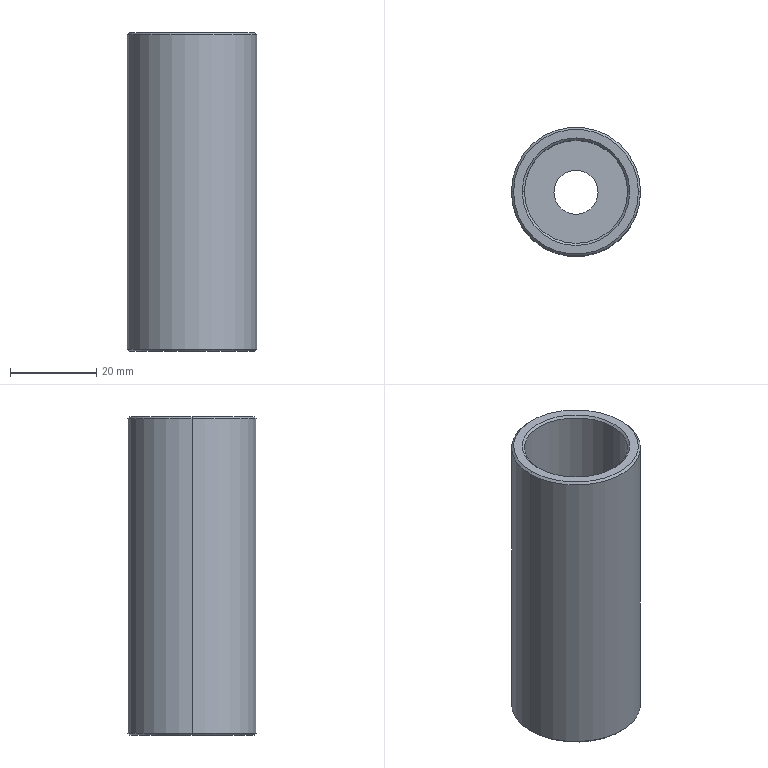Part | STEP file | Bucha guia BPR - BPR24074 | 1 solid | 15 faces | box 30 x 30 x 74 mm | volume 24346 mm3 | cone 6 | cylinder 6 | plane 3 | commonest cylinder face diameters 10.25 x2 24 x2 30 x2
STEP:
#1=CARTESIAN_POINT('',(0.,0.,0.));
#2=DIRECTION('',(0.,0.,1.));
#3=DIRECTION('',(1.,0.,0.));
#4=AXIS2_PLACEMENT_3D('',#1,#2,#3);
#5=CARTESIAN_POINT('',(12.,0.,73.5));
#6=VERTEX_POINT('',#5);
#7=CARTESIAN_POINT('',(12.5,0.,74.));
#8=VERTEX_POINT('',#7);
#9=CARTESIAN_POINT('',(12.5,0.,74.));
#10=DIRECTION('',(0.7071,0.,0.7071));
#11=VECTOR('',#10,1.);
#12=LINE('',#9,#11);
#13=CARTESIAN_POINT('',(0.,0.,74.));
#14=DIRECTION('',(0.,0.,1.));
#15=DIRECTION('',(1.,0.,0.));
#16=AXIS2_PLACEMENT_3D('',#13,#14,#15);
#17=CONICAL_SURFACE('',#16,12.5,0.7854);
#18=CARTESIAN_POINT('',(6.283,0.));
#19=DIRECTION('',(0.,1.));
#20=VECTOR('',#19,1.);
#21=LINE('',#18,#20);
#22=(GEOMETRIC_REPRESENTATION_CONTEXT(2)PARAMETRIC_REPRESENTATION_CONTEXT()REPRESENTATION_CONTEXT('',''));
#23=DEFINITIONAL_REPRESENTATION('',(#21),#22);
#24=PCURVE('',#17,#23);
#25=CARTESIAN_POINT('',(0.,0.,74.));
#26=DIRECTION('',(0.,0.,1.));
#27=DIRECTION('',(1.,0.,0.));
#28=AXIS2_PLACEMENT_3D('',#25,#26,#27);
#29=CONICAL_SURFACE('',#28,12.5,0.7854);
#30=CARTESIAN_POINT('',(0.,0.));
#31=DIRECTION('',(0.,1.));
#32=VECTOR('',#31,1.);
#33=LINE('',#30,#32);
#34=(GEOMETRIC_REPRESENTATION_CONTEXT(2)PARAMETRIC_REPRESENTATION_CONTEXT()REPRESENTATION_CONTEXT('',''));
#35=DEFINITIONAL_REPRESENTATION('',(#33),#34);
#36=PCURVE('',#29,#35);
#37=SURFACE_CURVE('',#12,(#24,#36),.PCURVE_S1.);
#38=EDGE_CURVE('',#6,#8,#37,.T.);
#39=ORIENTED_EDGE('',*,*,#38,.T.);
#40=CARTESIAN_POINT('',(-12.5,0.,74.));
#41=VERTEX_POINT('',#40);
#42=CARTESIAN_POINT('',(0.,0.,74.));
#43=DIRECTION('',(0.,0.,-1.));
#44=DIRECTION('',(1.,0.,0.));
#45=AXIS2_PLACEMENT_3D('',#42,#43,#44);
#46=CIRCLE('',#45,12.5);
#47=CARTESIAN_POINT('',(6.283,0.));
#48=DIRECTION('',(-1.,0.));
#49=VECTOR('',#48,1.);
#50=LINE('',#47,#49);
#51=(GEOMETRIC_REPRESENTATION_CONTEXT(2)PARAMETRIC_REPRESENTATION_CONTEXT()REPRESENTATION_CONTEXT('',''));
#52=DEFINITIONAL_REPRESENTATION('',(#50),#51);
#53=PCURVE('',#17,#52);
#54=CARTESIAN_POINT('',(15.,0.,74.));
#55=DIRECTION('',(0.,0.,1.));
#56=DIRECTION('',(1.,0.,0.));
#57=AXIS2_PLACEMENT_3D('',#54,#55,#56);
#58=PLANE('',#57);
#59=CARTESIAN_POINT('',(-2.5,0.));
#60=CARTESIAN_POINT('',(-2.5,-21.651));
#61=CARTESIAN_POINT('',(-21.25,-10.825));
#62=CARTESIAN_POINT('',(-40.,0.));
#63=CARTESIAN_POINT('',(-21.25,10.825));
#64=CARTESIAN_POINT('',(-2.5,21.651));
#65=CARTESIAN_POINT('',(-2.5,0.));
#66=(BOUNDED_CURVE()B_SPLINE_CURVE(2,(#59,#60,#61,#62,#63,#64,#65),.UNSPECIFIED.,.T.,.F.)B_SPLINE_CURVE_WITH_KNOTS((1,2,2,2,2,1),(-2.094,0.,2.094,4.189,6.283,8.378),.UNSPECIFIED.)CURVE()GEOMETRIC_REPRESENTATION_ITEM()RATIONAL_B_SPLINE_CURVE((1.,0.5,1.,0.5,1.,0.5,1.))REPRESENTATION_ITEM(''));
#67=(GEOMETRIC_REPRESENTATION_CONTEXT(2)PARAMETRIC_REPRESENTATION_CONTEXT()REPRESENTATION_CONTEXT('',''));
#68=DEFINITIONAL_REPRESENTATION('',(#66),#67);
#69=PCURVE('',#58,#68);
#70=SURFACE_CURVE('',#46,(#53,#69),.PCURVE_S1.);
#71=EDGE_CURVE('',#8,#41,#70,.T.);
#72=ORIENTED_EDGE('',*,*,#71,.T.);
#73=CARTESIAN_POINT('',(-12.,0.,73.5));
#74=VERTEX_POINT('',#73);
#75=CARTESIAN_POINT('',(-12.5,0.,74.));
#76=DIRECTION('',(-0.7071,0.,0.7071));
#77=VECTOR('',#76,1.);
#78=LINE('',#75,#77);
#79=CARTESIAN_POINT('',(3.142,0.));
#80=DIRECTION('',(0.,1.));
#81=VECTOR('',#80,1.);
#82=LINE('',#79,#81);
#83=(GEOMETRIC_REPRESENTATION_CONTEXT(2)PARAMETRIC_REPRESENTATION_CONTEXT()REPRESENTATION_CONTEXT('',''));
#84=DEFINITIONAL_REPRESENTATION('',(#82),#83);
#85=PCURVE('',#17,#84);
#86=CARTESIAN_POINT('',(3.142,0.));
#87=DIRECTION('',(0.,1.));
#88=VECTOR('',#87,1.);
#89=LINE('',#86,#88);
#90=(GEOMETRIC_REPRESENTATION_CONTEXT(2)PARAMETRIC_REPRESENTATION_CONTEXT()REPRESENTATION_CONTEXT('',''));
#91=DEFINITIONAL_REPRESENTATION('',(#89),#90);
#92=PCURVE('',#29,#91);
#93=SURFACE_CURVE('',#78,(#85,#92),.PCURVE_S1.);
#94=EDGE_CURVE('',#74,#41,#93,.T.);
#95=ORIENTED_EDGE('',*,*,#94,.F.);
#96=CARTESIAN_POINT('',(0.,0.,73.5));
#97=DIRECTION('',(0.,0.,1.));
#98=DIRECTION('',(1.,0.,0.));
#99=AXIS2_PLACEMENT_3D('',#96,#97,#98);
#100=CIRCLE('',#99,12.);
#101=CARTESIAN_POINT('',(0.,-0.5));
#102=DIRECTION('',(1.,0.));
#103=VECTOR('',#102,1.);
#104=LINE('',#101,#103);
#105=(GEOMETRIC_REPRESENTATION_CONTEXT(2)PARAMETRIC_REPRESENTATION_CONTEXT()REPRESENTATION_CONTEXT('',''));
#106=DEFINITIONAL_REPRESENTATION('',(#104),#105);
#107=PCURVE('',#17,#106);
#108=CARTESIAN_POINT('',(0.,0.,15.));
#109=DIRECTION('',(0.,0.,1.));
#110=DIRECTION('',(1.,0.,0.));
#111=AXIS2_PLACEMENT_3D('',#108,#109,#110);
#112=CYLINDRICAL_SURFACE('',#111,12.);
#113=CARTESIAN_POINT('',(0.,58.5));
#114=DIRECTION('',(1.,0.));
#115=VECTOR('',#114,1.);
#116=LINE('',#113,#115);
#117=(GEOMETRIC_REPRESENTATION_CONTEXT(2)PARAMETRIC_REPRESENTATION_CONTEXT()REPRESENTATION_CONTEXT('',''));
#118=DEFINITIONAL_REPRESENTATION('',(#116),#117);
#119=PCURVE('',#112,#118);
#120=SURFACE_CURVE('',#100,(#107,#119),.PCURVE_S1.);
#121=EDGE_CURVE('',#74,#6,#120,.T.);
#122=ORIENTED_EDGE('',*,*,#121,.T.);
#123=EDGE_LOOP('',(#39,#72,#95,#122));
#124=FACE_BOUND('',#123,.F.);
#125=ADVANCED_FACE('',(#124),#17,.F.);
#126=CARTESIAN_POINT('',(14.5,0.,74.));
#127=VERTEX_POINT('',#126);
#128=CARTESIAN_POINT('',(-14.5,0.,74.));
#129=VERTEX_POINT('',#128);
#130=CARTESIAN_POINT('',(0.,0.,74.));
#131=DIRECTION('',(0.,0.,1.));
#132=DIRECTION('',(1.,0.,0.));
#133=AXIS2_PLACEMENT_3D('',#130,#131,#132);
#134=CIRCLE('',#133,14.5);
#135=CARTESIAN_POINT('',(0.,0.,73.5));
#136=DIRECTION('',(0.,0.,-1.));
#137=DIRECTION('',(-1.,0.,0.));
#138=AXIS2_PLACEMENT_3D('',#135,#136,#137);
#139=CONICAL_SURFACE('',#138,15.,0.7854);
#140=CARTESIAN_POINT('',(3.142,-0.5));
#141=DIRECTION('',(-1.,0.));
#142=VECTOR('',#141,1.);
#143=LINE('',#140,#142);
#144=(GEOMETRIC_REPRESENTATION_CONTEXT(2)PARAMETRIC_REPRESENTATION_CONTEXT()REPRESENTATION_CONTEXT('',''));
#145=DEFINITIONAL_REPRESENTATION('',(#143),#144);
#146=PCURVE('',#139,#145);
#147=CARTESIAN_POINT('',(-15.,0.));
#148=DIRECTION('',(1.,0.));
#149=AXIS2_PLACEMENT_2D('',#147,#148);
#150=CIRCLE('',#149,14.5);
#151=(GEOMETRIC_REPRESENTATION_CONTEXT(2)PARAMETRIC_REPRESENTATION_CONTEXT()REPRESENTATION_CONTEXT('',''));
#152=DEFINITIONAL_REPRESENTATION('',(#150),#151);
#153=PCURVE('',#58,#152);
#154=SURFACE_CURVE('',#134,(#146,#153),.PCURVE_S1.);
#155=EDGE_CURVE('',#127,#129,#154,.T.);
#156=ORIENTED_EDGE('',*,*,#155,.F.);
#157=CARTESIAN_POINT('',(15.,0.,73.5));
#158=VERTEX_POINT('',#157);
#159=CARTESIAN_POINT('',(15.,0.,73.5));
#160=DIRECTION('',(0.7071,0.,-0.7071));
#161=VECTOR('',#160,1.);
#162=LINE('',#159,#161);
#163=CARTESIAN_POINT('',(3.142,0.));
#164=DIRECTION('',(0.,1.));
#165=VECTOR('',#164,1.);
#166=LINE('',#163,#165);
#167=(GEOMETRIC_REPRESENTATION_CONTEXT(2)PARAMETRIC_REPRESENTATION_CONTEXT()REPRESENTATION_CONTEXT('',''));
#168=DEFINITIONAL_REPRESENTATION('',(#166),#167);
#169=PCURVE('',#139,#168);
#170=CARTESIAN_POINT('',(0.,0.,73.5));
#171=DIRECTION('',(0.,0.,-1.));
#172=DIRECTION('',(-1.,0.,0.));
#173=AXIS2_PLACEMENT_3D('',#170,#171,#172);
#174=CONICAL_SURFACE('',#173,15.,0.7854);
#175=CARTESIAN_POINT('',(3.142,0.));
#176=DIRECTION('',(0.,1.));
#177=VECTOR('',#176,1.);
#178=LINE('',#175,#177);
#179=(GEOMETRIC_REPRESENTATION_CONTEXT(2)PARAMETRIC_REPRESENTATION_CONTEXT()REPRESENTATION_CONTEXT('',''));
#180=DEFINITIONAL_REPRESENTATION('',(#178),#179);
#181=PCURVE('',#174,#180);
#182=SURFACE_CURVE('',#162,(#169,#181),.PCURVE_S1.);
#183=EDGE_CURVE('',#127,#158,#182,.T.);
#184=ORIENTED_EDGE('',*,*,#183,.T.);
#185=CARTESIAN_POINT('',(-15.,0.,73.5));
#186=VERTEX_POINT('',#185);
#187=CARTESIAN_POINT('',(0.,0.,73.5));
#188=DIRECTION('',(0.,0.,-1.));
#189=DIRECTION('',(1.,0.,0.));
#190=AXIS2_PLACEMENT_3D('',#187,#188,#189);
#191=CIRCLE('',#190,15.);
#192=CARTESIAN_POINT('',(-3.142,0.));
#193=DIRECTION('',(1.,0.));
#194=VECTOR('',#193,1.);
#195=LINE('',#192,#194);
#196=(GEOMETRIC_REPRESENTATION_CONTEXT(2)PARAMETRIC_REPRESENTATION_CONTEXT()REPRESENTATION_CONTEXT('',''));
#197=DEFINITIONAL_REPRESENTATION('',(#195),#196);
#198=PCURVE('',#139,#197);
#199=CARTESIAN_POINT('',(0.,0.,0.));
#200=DIRECTION('',(0.,0.,-1.));
#201=DIRECTION('',(-1.,0.,0.));
#202=AXIS2_PLACEMENT_3D('',#199,#200,#201);
#203=CYLINDRICAL_SURFACE('',#202,15.);
#204=CARTESIAN_POINT('',(-3.142,-73.5));
#205=DIRECTION('',(1.,0.));
#206=VECTOR('',#205,1.);
#207=LINE('',#204,#206);
#208=(GEOMETRIC_REPRESENTATION_CONTEXT(2)PARAMETRIC_REPRESENTATION_CONTEXT()REPRESENTATION_CONTEXT('',''));
#209=DEFINITIONAL_REPRESENTATION('',(#207),#208);
#210=PCURVE('',#203,#209);
#211=SURFACE_CURVE('',#191,(#198,#210),.PCURVE_S1.);
#212=EDGE_CURVE('',#186,#158,#211,.T.);
#213=ORIENTED_EDGE('',*,*,#212,.F.);
#214=CARTESIAN_POINT('',(-15.,0.,73.5));
#215=DIRECTION('',(-0.7071,0.,-0.7071));
#216=VECTOR('',#215,1.);
#217=LINE('',#214,#216);
#218=CARTESIAN_POINT('',(0.,0.));
#219=DIRECTION('',(0.,1.));
#220=VECTOR('',#219,1.);
#221=LINE('',#218,#220);
#222=(GEOMETRIC_REPRESENTATION_CONTEXT(2)PARAMETRIC_REPRESENTATION_CONTEXT()REPRESENTATION_CONTEXT('',''));
#223=DEFINITIONAL_REPRESENTATION('',(#221),#222);
#224=PCURVE('',#139,#223);
#225=CARTESIAN_POINT('',(6.283,0.));
#226=DIRECTION('',(0.,1.));
#227=VECTOR('',#226,1.);
#228=LINE('',#225,#227);
#229=(GEOMETRIC_REPRESENTATION_CONTEXT(2)PARAMETRIC_REPRESENTATION_CONTEXT()REPRESENTATION_CONTEXT('',''));
#230=DEFINITIONAL_REPRESENTATION('',(#228),#229);
#231=PCURVE('',#174,#230);
#232=SURFACE_CURVE('',#217,(#224,#231),.PCURVE_S1.);
#233=EDGE_CURVE('',#129,#186,#232,.T.);
#234=ORIENTED_EDGE('',*,*,#233,.F.);
#235=EDGE_LOOP('',(#156,#184,#213,#234));
#236=FACE_BOUND('',#235,.T.);
#237=ADVANCED_FACE('',(#236),#139,.T.);
#238=CARTESIAN_POINT('',(-14.5,0.,0.));
#239=VERTEX_POINT('',#238);
#240=CARTESIAN_POINT('',(14.5,0.,0.));
#241=VERTEX_POINT('',#240);
#242=CARTESIAN_POINT('',(0.,0.,0.));
#243=DIRECTION('',(0.,0.,-1.));
#244=DIRECTION('',(-1.,0.,0.));
#245=AXIS2_PLACEMENT_3D('',#242,#243,#244);
#246=CIRCLE('',#245,14.5);
#247=CARTESIAN_POINT('',(0.,0.,0.));
#248=DIRECTION('',(0.,0.,1.));
#249=DIRECTION('',(1.,0.,0.));
#250=AXIS2_PLACEMENT_3D('',#247,#248,#249);
#251=CONICAL_SURFACE('',#250,14.5,0.7854);
#252=CARTESIAN_POINT('',(3.142,0.));
#253=DIRECTION('',(-1.,0.));
#254=VECTOR('',#253,1.);
#255=LINE('',#252,#254);
#256=(GEOMETRIC_REPRESENTATION_CONTEXT(2)PARAMETRIC_REPRESENTATION_CONTEXT()REPRESENTATION_CONTEXT('',''));
#257=DEFINITIONAL_REPRESENTATION('',(#255),#256);
#258=PCURVE('',#251,#257);
#259=CARTESIAN_POINT('',(0.,0.,0.));
#260=DIRECTION('',(0.,0.,-1.));
#261=DIRECTION('',(-1.,0.,0.));
#262=AXIS2_PLACEMENT_3D('',#259,#260,#261);
#263=PLANE('',#262);
#264=CARTESIAN_POINT('',(0.,0.));
#265=DIRECTION('',(1.,0.));
#266=AXIS2_PLACEMENT_2D('',#264,#265);
#267=CIRCLE('',#266,14.5);
#268=(GEOMETRIC_REPRESENTATION_CONTEXT(2)PARAMETRIC_REPRESENTATION_CONTEXT()REPRESENTATION_CONTEXT('',''));
#269=DEFINITIONAL_REPRESENTATION('',(#267),#268);
#270=PCURVE('',#263,#269);
#271=SURFACE_CURVE('',#246,(#258,#270),.PCURVE_S1.);
#272=EDGE_CURVE('',#239,#241,#271,.T.);
#273=ORIENTED_EDGE('',*,*,#272,.F.);
#274=CARTESIAN_POINT('',(-15.,0.,0.5));
#275=VERTEX_POINT('',#274);
#276=CARTESIAN_POINT('',(-14.5,0.,0.));
#277=DIRECTION('',(-0.7071,0.,0.7071));
#278=VECTOR('',#277,1.);
#279=LINE('',#276,#278);
#280=CARTESIAN_POINT('',(3.142,0.));
#281=DIRECTION('',(0.,1.));
#282=VECTOR('',#281,1.);
#283=LINE('',#280,#282);
#284=(GEOMETRIC_REPRESENTATION_CONTEXT(2)PARAMETRIC_REPRESENTATION_CONTEXT()REPRESENTATION_CONTEXT('',''));
#285=DEFINITIONAL_REPRESENTATION('',(#283),#284);
#286=PCURVE('',#251,#285);
#287=CARTESIAN_POINT('',(0.,0.,0.));
#288=DIRECTION('',(0.,0.,1.));
#289=DIRECTION('',(1.,0.,0.));
#290=AXIS2_PLACEMENT_3D('',#287,#288,#289);
#291=CONICAL_SURFACE('',#290,14.5,0.7854);
#292=CARTESIAN_POINT('',(3.142,0.));
#293=DIRECTION('',(0.,1.));
#294=VECTOR('',#293,1.);
#295=LINE('',#292,#294);
#296=(GEOMETRIC_REPRESENTATION_CONTEXT(2)PARAMETRIC_REPRESENTATION_CONTEXT()REPRESENTATION_CONTEXT('',''));
#297=DEFINITIONAL_REPRESENTATION('',(#295),#296);
#298=PCURVE('',#291,#297);
#299=SURFACE_CURVE('',#279,(#286,#298),.PCURVE_S1.);
#300=EDGE_CURVE('',#239,#275,#299,.T.);
#301=ORIENTED_EDGE('',*,*,#300,.T.);
#302=CARTESIAN_POINT('',(15.,0.,0.5));
#303=VERTEX_POINT('',#302);
#304=CARTESIAN_POINT('',(0.,0.,0.5));
#305=DIRECTION('',(0.,0.,1.));
#306=DIRECTION('',(-1.,0.,0.));
#307=AXIS2_PLACEMENT_3D('',#304,#305,#306);
#308=CIRCLE('',#307,15.);
#309=CARTESIAN_POINT('',(-3.142,0.5));
#310=DIRECTION('',(1.,0.));
#311=VECTOR('',#310,1.);
#312=LINE('',#309,#311);
#313=(GEOMETRIC_REPRESENTATION_CONTEXT(2)PARAMETRIC_REPRESENTATION_CONTEXT()REPRESENTATION_CONTEXT('',''));
#314=DEFINITIONAL_REPRESENTATION('',(#312),#313);
#315=PCURVE('',#251,#314);
#316=CARTESIAN_POINT('',(6.283,-0.5));
#317=DIRECTION('',(-1.,0.));
#318=VECTOR('',#317,1.);
#319=LINE('',#316,#318);
#320=(GEOMETRIC_REPRESENTATION_CONTEXT(2)PARAMETRIC_REPRESENTATION_CONTEXT()REPRESENTATION_CONTEXT('',''));
#321=DEFINITIONAL_REPRESENTATION('',(#319),#320);
#322=PCURVE('',#203,#321);
#323=SURFACE_CURVE('',#308,(#315,#322),.PCURVE_S1.);
#324=EDGE_CURVE('',#303,#275,#323,.T.);
#325=ORIENTED_EDGE('',*,*,#324,.F.);
#326=CARTESIAN_POINT('',(14.5,0.,0.));
#327=DIRECTION('',(0.7071,0.,0.7071));
#328=VECTOR('',#327,1.);
#329=LINE('',#326,#328);
#330=CARTESIAN_POINT('',(0.,0.));
#331=DIRECTION('',(0.,1.));
#332=VECTOR('',#331,1.);
#333=LINE('',#330,#332);
#334=(GEOMETRIC_REPRESENTATION_CONTEXT(2)PARAMETRIC_REPRESENTATION_CONTEXT()REPRESENTATION_CONTEXT('',''));
#335=DEFINITIONAL_REPRESENTATION('',(#333),#334);
#336=PCURVE('',#251,#335);
#337=CARTESIAN_POINT('',(6.283,0.));
#338=DIRECTION('',(0.,1.));
#339=VECTOR('',#338,1.);
#340=LINE('',#337,#339);
#341=(GEOMETRIC_REPRESENTATION_CONTEXT(2)PARAMETRIC_REPRESENTATION_CONTEXT()REPRESENTATION_CONTEXT('',''));
#342=DEFINITIONAL_REPRESENTATION('',(#340),#341);
#343=PCURVE('',#291,#342);
#344=SURFACE_CURVE('',#329,(#336,#343),.PCURVE_S1.);
#345=EDGE_CURVE('',#241,#303,#344,.T.);
#346=ORIENTED_EDGE('',*,*,#345,.F.);
#347=EDGE_LOOP('',(#273,#301,#325,#346));
#348=FACE_BOUND('',#347,.T.);
#349=ADVANCED_FACE('',(#348),#251,.T.);
#350=CARTESIAN_POINT('',(12.,0.,15.));
#351=VERTEX_POINT('',#350);
#352=CARTESIAN_POINT('',(12.,0.,15.));
#353=DIRECTION('',(0.,0.,1.));
#354=VECTOR('',#353,1.);
#355=LINE('',#352,#354);
#356=CARTESIAN_POINT('',(6.283,0.));
#357=DIRECTION('',(0.,1.));
#358=VECTOR('',#357,1.);
#359=LINE('',#356,#358);
#360=(GEOMETRIC_REPRESENTATION_CONTEXT(2)PARAMETRIC_REPRESENTATION_CONTEXT()REPRESENTATION_CONTEXT('',''));
#361=DEFINITIONAL_REPRESENTATION('',(#359),#360);
#362=PCURVE('',#112,#361);
#363=CARTESIAN_POINT('',(0.,0.,15.));
#364=DIRECTION('',(0.,0.,1.));
#365=DIRECTION('',(1.,0.,0.));
#366=AXIS2_PLACEMENT_3D('',#363,#364,#365);
#367=CYLINDRICAL_SURFACE('',#366,12.);
#368=CARTESIAN_POINT('',(0.,0.));
#369=DIRECTION('',(0.,1.));
#370=VECTOR('',#369,1.);
#371=LINE('',#368,#370);
#372=(GEOMETRIC_REPRESENTATION_CONTEXT(2)PARAMETRIC_REPRESENTATION_CONTEXT()REPRESENTATION_CONTEXT('',''));
#373=DEFINITIONAL_REPRESENTATION('',(#371),#372);
#374=PCURVE('',#367,#373);
#375=SURFACE_CURVE('',#355,(#362,#374),.PCURVE_S1.);
#376=EDGE_CURVE('',#351,#6,#375,.T.);
#377=ORIENTED_EDGE('',*,*,#376,.T.);
#378=ORIENTED_EDGE('',*,*,#121,.F.);
#379=CARTESIAN_POINT('',(-12.,0.,15.));
#380=VERTEX_POINT('',#379);
#381=CARTESIAN_POINT('',(-12.,0.,15.));
#382=DIRECTION('',(0.,0.,1.));
#383=VECTOR('',#382,1.);
#384=LINE('',#381,#383);
#385=CARTESIAN_POINT('',(3.142,0.));
#386=DIRECTION('',(0.,1.));
#387=VECTOR('',#386,1.);
#388=LINE('',#385,#387);
#389=(GEOMETRIC_REPRESENTATION_CONTEXT(2)PARAMETRIC_REPRESENTATION_CONTEXT()REPRESENTATION_CONTEXT('',''));
#390=DEFINITIONAL_REPRESENTATION('',(#388),#389);
#391=PCURVE('',#112,#390);
#392=CARTESIAN_POINT('',(3.142,0.));
#393=DIRECTION('',(0.,1.));
#394=VECTOR('',#393,1.);
#395=LINE('',#392,#394);
#396=(GEOMETRIC_REPRESENTATION_CONTEXT(2)PARAMETRIC_REPRESENTATION_CONTEXT()REPRESENTATION_CONTEXT('',''));
#397=DEFINITIONAL_REPRESENTATION('',(#395),#396);
#398=PCURVE('',#367,#397);
#399=SURFACE_CURVE('',#384,(#391,#398),.PCURVE_S1.);
#400=EDGE_CURVE('',#380,#74,#399,.T.);
#401=ORIENTED_EDGE('',*,*,#400,.F.);
#402=CARTESIAN_POINT('',(0.,0.,15.));
#403=DIRECTION('',(0.,0.,1.));
#404=DIRECTION('',(1.,0.,0.));
#405=AXIS2_PLACEMENT_3D('',#402,#403,#404);
#406=CIRCLE('',#405,12.);
#407=CARTESIAN_POINT('',(0.,0.));
#408=DIRECTION('',(1.,0.));
#409=VECTOR('',#408,1.);
#410=LINE('',#407,#409);
#411=(GEOMETRIC_REPRESENTATION_CONTEXT(2)PARAMETRIC_REPRESENTATION_CONTEXT()REPRESENTATION_CONTEXT('',''));
#412=DEFINITIONAL_REPRESENTATION('',(#410),#411);
#413=PCURVE('',#112,#412);
#414=CARTESIAN_POINT('',(0.,0.,15.));
#415=DIRECTION('',(0.,0.,-1.));
#416=DIRECTION('',(-1.,0.,0.));
#417=AXIS2_PLACEMENT_3D('',#414,#415,#416);
#418=PLANE('',#417);
#419=CARTESIAN_POINT('',(-12.,0.));
#420=CARTESIAN_POINT('',(-12.,20.785));
#421=CARTESIAN_POINT('',(6.,10.392));
#422=CARTESIAN_POINT('',(24.,0.));
#423=CARTESIAN_POINT('',(6.,-10.392));
#424=CARTESIAN_POINT('',(-12.,-20.785));
#425=CARTESIAN_POINT('',(-12.,0.));
#426=(BOUNDED_CURVE()B_SPLINE_CURVE(2,(#419,#420,#421,#422,#423,#424,#425),.UNSPECIFIED.,.T.,.F.)B_SPLINE_CURVE_WITH_KNOTS((1,2,2,2,2,1),(-2.094,0.,2.094,4.189,6.283,8.378),.UNSPECIFIED.)CURVE()GEOMETRIC_REPRESENTATION_ITEM()RATIONAL_B_SPLINE_CURVE((1.,0.5,1.,0.5,1.,0.5,1.))REPRESENTATION_ITEM(''));
#427=(GEOMETRIC_REPRESENTATION_CONTEXT(2)PARAMETRIC_REPRESENTATION_CONTEXT()REPRESENTATION_CONTEXT('',''));
#428=DEFINITIONAL_REPRESENTATION('',(#426),#427);
#429=PCURVE('',#418,#428);
#430=SURFACE_CURVE('',#406,(#413,#429),.PCURVE_S1.);
#431=EDGE_CURVE('',#380,#351,#430,.T.);
#432=ORIENTED_EDGE('',*,*,#431,.T.);
#433=EDGE_LOOP('',(#377,#378,#401,#432));
#434=FACE_BOUND('',#433,.F.);
#435=ADVANCED_FACE('',(#434),#112,.F.);
#436=CARTESIAN_POINT('',(5.125,0.,15.));
#437=VERTEX_POINT('',#436);
#438=CARTESIAN_POINT('',(5.125,0.,0.));
#439=VERTEX_POINT('',#438);
#440=CARTESIAN_POINT('',(5.125,0.,23.75));
#441=DIRECTION('',(0.,0.,-1.));
#442=VECTOR('',#441,1.);
#443=LINE('',#440,#442);
#444=CARTESIAN_POINT('',(0.,0.,23.75));
#445=DIRECTION('',(0.,0.,-1.));
#446=DIRECTION('',(1.,0.,0.));
#447=AXIS2_PLACEMENT_3D('',#444,#445,#446);
#448=CYLINDRICAL_SURFACE('',#447,5.125);
#449=CARTESIAN_POINT('',(6.283,0.));
#450=DIRECTION('',(0.,1.));
#451=VECTOR('',#450,1.);
#452=LINE('',#449,#451);
#453=(GEOMETRIC_REPRESENTATION_CONTEXT(2)PARAMETRIC_REPRESENTATION_CONTEXT()REPRESENTATION_CONTEXT('',''));
#454=DEFINITIONAL_REPRESENTATION('',(#452),#453);
#455=PCURVE('',#448,#454);
#456=CARTESIAN_POINT('',(0.,0.,23.75));
#457=DIRECTION('',(0.,0.,-1.));
#458=DIRECTION('',(1.,0.,0.));
#459=AXIS2_PLACEMENT_3D('',#456,#457,#458);
#460=CYLINDRICAL_SURFACE('',#459,5.125);
#461=CARTESIAN_POINT('',(0.,0.));
#462=DIRECTION('',(0.,1.));
#463=VECTOR('',#462,1.);
#464=LINE('',#461,#463);
#465=(GEOMETRIC_REPRESENTATION_CONTEXT(2)PARAMETRIC_REPRESENTATION_CONTEXT()REPRESENTATION_CONTEXT('',''));
#466=DEFINITIONAL_REPRESENTATION('',(#464),#465);
#467=PCURVE('',#460,#466);
#468=SURFACE_CURVE('',#443,(#455,#467),.PCURVE_S1.);
#469=EDGE_CURVE('',#437,#439,#468,.T.);
#470=ORIENTED_EDGE('',*,*,#469,.T.);
#471=CARTESIAN_POINT('',(-5.125,0.,0.));
#472=VERTEX_POINT('',#471);
#473=CARTESIAN_POINT('',(0.,0.,0.));
#474=DIRECTION('',(0.,0.,1.));
#475=DIRECTION('',(1.,0.,0.));
#476=AXIS2_PLACEMENT_3D('',#473,#474,#475);
#477=CIRCLE('',#476,5.125);
#478=CARTESIAN_POINT('',(6.283,23.75));
#479=DIRECTION('',(-1.,0.));
#480=VECTOR('',#479,1.);
#481=LINE('',#478,#480);
#482=(GEOMETRIC_REPRESENTATION_CONTEXT(2)PARAMETRIC_REPRESENTATION_CONTEXT()REPRESENTATION_CONTEXT('',''));
#483=DEFINITIONAL_REPRESENTATION('',(#481),#482);
#484=PCURVE('',#448,#483);
#485=CARTESIAN_POINT('',(-5.125,0.));
#486=CARTESIAN_POINT('',(-5.125,8.877));
#487=CARTESIAN_POINT('',(2.562,4.438));
#488=CARTESIAN_POINT('',(10.25,0.));
#489=CARTESIAN_POINT('',(2.562,-4.438));
#490=CARTESIAN_POINT('',(-5.125,-8.877));
#491=CARTESIAN_POINT('',(-5.125,0.));
#492=(BOUNDED_CURVE()B_SPLINE_CURVE(2,(#485,#486,#487,#488,#489,#490,#491),.UNSPECIFIED.,.T.,.F.)B_SPLINE_CURVE_WITH_KNOTS((1,2,2,2,2,1),(-2.094,0.,2.094,4.189,6.283,8.378),.UNSPECIFIED.)CURVE()GEOMETRIC_REPRESENTATION_ITEM()RATIONAL_B_SPLINE_CURVE((1.,0.5,1.,0.5,1.,0.5,1.))REPRESENTATION_ITEM(''));
#493=(GEOMETRIC_REPRESENTATION_CONTEXT(2)PARAMETRIC_REPRESENTATION_CONTEXT()REPRESENTATION_CONTEXT('',''));
#494=DEFINITIONAL_REPRESENTATION('',(#492),#493);
#495=PCURVE('',#263,#494);
#496=SURFACE_CURVE('',#477,(#484,#495),.PCURVE_S1.);
#497=EDGE_CURVE('',#439,#472,#496,.T.);
#498=ORIENTED_EDGE('',*,*,#497,.T.);
#499=CARTESIAN_POINT('',(-5.125,0.,15.));
#500=VERTEX_POINT('',#499);
#501=CARTESIAN_POINT('',(-5.125,0.,23.75));
#502=DIRECTION('',(0.,0.,-1.));
#503=VECTOR('',#502,1.);
#504=LINE('',#501,#503);
#505=CARTESIAN_POINT('',(3.142,0.));
#506=DIRECTION('',(0.,1.));
#507=VECTOR('',#506,1.);
#508=LINE('',#505,#507);
#509=(GEOMETRIC_REPRESENTATION_CONTEXT(2)PARAMETRIC_REPRESENTATION_CONTEXT()REPRESENTATION_CONTEXT('',''));
#510=DEFINITIONAL_REPRESENTATION('',(#508),#509);
#511=PCURVE('',#448,#510);
#512=CARTESIAN_POINT('',(3.142,0.));
#513=DIRECTION('',(0.,1.));
#514=VECTOR('',#513,1.);
#515=LINE('',#512,#514);
#516=(GEOMETRIC_REPRESENTATION_CONTEXT(2)PARAMETRIC_REPRESENTATION_CONTEXT()REPRESENTATION_CONTEXT('',''));
#517=DEFINITIONAL_REPRESENTATION('',(#515),#516);
#518=PCURVE('',#460,#517);
#519=SURFACE_CURVE('',#504,(#511,#518),.PCURVE_S1.);
#520=EDGE_CURVE('',#500,#472,#519,.T.);
#521=ORIENTED_EDGE('',*,*,#520,.F.);
#522=CARTESIAN_POINT('',(0.,0.,15.));
#523=DIRECTION('',(0.,0.,1.));
#524=DIRECTION('',(-1.,0.,0.));
#525=AXIS2_PLACEMENT_3D('',#522,#523,#524);
#526=CIRCLE('',#525,5.125);
#527=CARTESIAN_POINT('',(9.425,8.75));
#528=DIRECTION('',(-1.,0.));
#529=VECTOR('',#528,1.);
#530=LINE('',#527,#529);
#531=(GEOMETRIC_REPRESENTATION_CONTEXT(2)PARAMETRIC_REPRESENTATION_CONTEXT()REPRESENTATION_CONTEXT('',''));
#532=DEFINITIONAL_REPRESENTATION('',(#530),#531);
#533=PCURVE('',#448,#532);
#534=CARTESIAN_POINT('',(5.125,0.));
#535=CARTESIAN_POINT('',(5.125,-8.877));
#536=CARTESIAN_POINT('',(-2.562,-4.438));
#537=CARTESIAN_POINT('',(-10.25,0.));
#538=CARTESIAN_POINT('',(-2.562,4.438));
#539=CARTESIAN_POINT('',(5.125,8.877));
#540=CARTESIAN_POINT('',(5.125,0.));
#541=(BOUNDED_CURVE()B_SPLINE_CURVE(2,(#534,#535,#536,#537,#538,#539,#540),.UNSPECIFIED.,.T.,.F.)B_SPLINE_CURVE_WITH_KNOTS((1,2,2,2,2,1),(-2.094,0.,2.094,4.189,6.283,8.378),.UNSPECIFIED.)CURVE()GEOMETRIC_REPRESENTATION_ITEM()RATIONAL_B_SPLINE_CURVE((1.,0.5,1.,0.5,1.,0.5,1.))REPRESENTATION_ITEM(''));
#542=(GEOMETRIC_REPRESENTATION_CONTEXT(2)PARAMETRIC_REPRESENTATION_CONTEXT()REPRESENTATION_CONTEXT('',''));
#543=DEFINITIONAL_REPRESENTATION('',(#541),#542);
#544=PCURVE('',#418,#543);
#545=SURFACE_CURVE('',#526,(#533,#544),.PCURVE_S1.);
#546=EDGE_CURVE('',#437,#500,#545,.T.);
#547=ORIENTED_EDGE('',*,*,#546,.F.);
#548=EDGE_LOOP('',(#470,#498,#521,#547));
#549=FACE_BOUND('',#548,.F.);
#550=ADVANCED_FACE('',(#549),#448,.F.);
#551=ORIENTED_EDGE('',*,*,#212,.T.);
#552=CARTESIAN_POINT('',(15.,0.,0.));
#553=DIRECTION('',(0.,0.,-1.));
#554=VECTOR('',#553,1.);
#555=LINE('',#552,#554);
#556=CARTESIAN_POINT('',(3.142,0.));
#557=DIRECTION('',(0.,1.));
#558=VECTOR('',#557,1.);
#559=LINE('',#556,#558);
#560=(GEOMETRIC_REPRESENTATION_CONTEXT(2)PARAMETRIC_REPRESENTATION_CONTEXT()REPRESENTATION_CONTEXT('',''));
#561=DEFINITIONAL_REPRESENTATION('',(#559),#560);
#562=PCURVE('',#203,#561);
#563=CARTESIAN_POINT('',(0.,0.,0.));
#564=DIRECTION('',(0.,0.,-1.));
#565=DIRECTION('',(-1.,0.,0.));
#566=AXIS2_PLACEMENT_3D('',#563,#564,#565);
#567=CYLINDRICAL_SURFACE('',#566,15.);
#568=CARTESIAN_POINT('',(3.142,0.));
#569=DIRECTION('',(0.,1.));
#570=VECTOR('',#569,1.);
#571=LINE('',#568,#570);
#572=(GEOMETRIC_REPRESENTATION_CONTEXT(2)PARAMETRIC_REPRESENTATION_CONTEXT()REPRESENTATION_CONTEXT('',''));
#573=DEFINITIONAL_REPRESENTATION('',(#571),#572);
#574=PCURVE('',#567,#573);
#575=SURFACE_CURVE('',#555,(#562,#574),.PCURVE_S1.);
#576=EDGE_CURVE('',#158,#303,#575,.T.);
#577=ORIENTED_EDGE('',*,*,#576,.T.);
#578=ORIENTED_EDGE('',*,*,#324,.T.);
#579=CARTESIAN_POINT('',(-15.,0.,0.));
#580=DIRECTION('',(0.,0.,-1.));
#581=VECTOR('',#580,1.);
#582=LINE('',#579,#581);
#583=CARTESIAN_POINT('',(0.,0.));
#584=DIRECTION('',(0.,1.));
#585=VECTOR('',#584,1.);
#586=LINE('',#583,#585);
#587=(GEOMETRIC_REPRESENTATION_CONTEXT(2)PARAMETRIC_REPRESENTATION_CONTEXT()REPRESENTATION_CONTEXT('',''));
#588=DEFINITIONAL_REPRESENTATION('',(#586),#587);
#589=PCURVE('',#203,#588);
#590=CARTESIAN_POINT('',(6.283,0.));
#591=DIRECTION('',(0.,1.));
#592=VECTOR('',#591,1.);
#593=LINE('',#590,#592);
#594=(GEOMETRIC_REPRESENTATION_CONTEXT(2)PARAMETRIC_REPRESENTATION_CONTEXT()REPRESENTATION_CONTEXT('',''));
#595=DEFINITIONAL_REPRESENTATION('',(#593),#594);
#596=PCURVE('',#567,#595);
#597=SURFACE_CURVE('',#582,(#589,#596),.PCURVE_S1.);
#598=EDGE_CURVE('',#186,#275,#597,.T.);
#599=ORIENTED_EDGE('',*,*,#598,.F.);
#600=EDGE_LOOP('',(#551,#577,#578,#599));
#601=FACE_BOUND('',#600,.T.);
#602=ADVANCED_FACE('',(#601),#203,.T.);
#603=CARTESIAN_POINT('',(0.,0.,0.));
#604=DIRECTION('',(0.,0.,-1.));
#605=DIRECTION('',(-1.,0.,0.));
#606=AXIS2_PLACEMENT_3D('',#603,#604,#605);
#607=CIRCLE('',#606,14.5);
#608=CARTESIAN_POINT('',(0.,0.));
#609=DIRECTION('',(1.,0.));
#610=AXIS2_PLACEMENT_2D('',#608,#609);
#611=CIRCLE('',#610,14.5);
#612=(GEOMETRIC_REPRESENTATION_CONTEXT(2)PARAMETRIC_REPRESENTATION_CONTEXT()REPRESENTATION_CONTEXT('',''));
#613=DEFINITIONAL_REPRESENTATION('',(#611),#612);
#614=PCURVE('',#263,#613);
#615=CARTESIAN_POINT('',(9.425,0.));
#616=DIRECTION('',(-1.,0.));
#617=VECTOR('',#616,1.);
#618=LINE('',#615,#617);
#619=(GEOMETRIC_REPRESENTATION_CONTEXT(2)PARAMETRIC_REPRESENTATION_CONTEXT()REPRESENTATION_CONTEXT('',''));
#620=DEFINITIONAL_REPRESENTATION('',(#618),#619);
#621=PCURVE('',#291,#620);
#622=SURFACE_CURVE('',#607,(#614,#621),.PCURVE_S1.);
#623=EDGE_CURVE('',#241,#239,#622,.T.);
#624=ORIENTED_EDGE('',*,*,#623,.T.);
#625=ORIENTED_EDGE('',*,*,#272,.T.);
#626=EDGE_LOOP('',(#624,#625));
#627=FACE_BOUND('',#626,.T.);
#628=ORIENTED_EDGE('',*,*,#497,.T.);
#629=CARTESIAN_POINT('',(0.,0.,0.));
#630=DIRECTION('',(0.,0.,1.));
#631=DIRECTION('',(1.,0.,0.));
#632=AXIS2_PLACEMENT_3D('',#629,#630,#631);
#633=CIRCLE('',#632,5.125);
#634=CARTESIAN_POINT('',(-5.125,0.));
#635=CARTESIAN_POINT('',(-5.125,8.877));
#636=CARTESIAN_POINT('',(2.562,4.438));
#637=CARTESIAN_POINT('',(10.25,0.));
#638=CARTESIAN_POINT('',(2.562,-4.438));
#639=CARTESIAN_POINT('',(-5.125,-8.877));
#640=CARTESIAN_POINT('',(-5.125,0.));
#641=(BOUNDED_CURVE()B_SPLINE_CURVE(2,(#634,#635,#636,#637,#638,#639,#640),.UNSPECIFIED.,.T.,.F.)B_SPLINE_CURVE_WITH_KNOTS((1,2,2,2,2,1),(-2.094,0.,2.094,4.189,6.283,8.378),.UNSPECIFIED.)CURVE()GEOMETRIC_REPRESENTATION_ITEM()RATIONAL_B_SPLINE_CURVE((1.,0.5,1.,0.5,1.,0.5,1.))REPRESENTATION_ITEM(''));
#642=(GEOMETRIC_REPRESENTATION_CONTEXT(2)PARAMETRIC_REPRESENTATION_CONTEXT()REPRESENTATION_CONTEXT('',''));
#643=DEFINITIONAL_REPRESENTATION('',(#641),#642);
#644=PCURVE('',#263,#643);
#645=CARTESIAN_POINT('',(6.283,23.75));
#646=DIRECTION('',(-1.,0.));
#647=VECTOR('',#646,1.);
#648=LINE('',#645,#647);
#649=(GEOMETRIC_REPRESENTATION_CONTEXT(2)PARAMETRIC_REPRESENTATION_CONTEXT()REPRESENTATION_CONTEXT('',''));
#650=DEFINITIONAL_REPRESENTATION('',(#648),#649);
#651=PCURVE('',#460,#650);
#652=SURFACE_CURVE('',#633,(#644,#651),.PCURVE_S1.);
#653=EDGE_CURVE('',#472,#439,#652,.T.);
#654=ORIENTED_EDGE('',*,*,#653,.T.);
#655=EDGE_LOOP('',(#628,#654));
#656=FACE_BOUND('',#655,.T.);
#657=ADVANCED_FACE('',(#627,#656),#263,.T.);
#658=ORIENTED_EDGE('',*,*,#576,.F.);
#659=CARTESIAN_POINT('',(0.,0.,73.5));
#660=DIRECTION('',(0.,0.,-1.));
#661=DIRECTION('',(1.,0.,0.));
#662=AXIS2_PLACEMENT_3D('',#659,#660,#661);
#663=CIRCLE('',#662,15.);
#664=CARTESIAN_POINT('',(3.142,-73.5));
#665=DIRECTION('',(1.,0.));
#666=VECTOR('',#665,1.);
#667=LINE('',#664,#666);
#668=(GEOMETRIC_REPRESENTATION_CONTEXT(2)PARAMETRIC_REPRESENTATION_CONTEXT()REPRESENTATION_CONTEXT('',''));
#669=DEFINITIONAL_REPRESENTATION('',(#667),#668);
#670=PCURVE('',#567,#669);
#671=CARTESIAN_POINT('',(3.142,0.));
#672=DIRECTION('',(1.,0.));
#673=VECTOR('',#672,1.);
#674=LINE('',#671,#673);
#675=(GEOMETRIC_REPRESENTATION_CONTEXT(2)PARAMETRIC_REPRESENTATION_CONTEXT()REPRESENTATION_CONTEXT('',''));
#676=DEFINITIONAL_REPRESENTATION('',(#674),#675);
#677=PCURVE('',#174,#676);
#678=SURFACE_CURVE('',#663,(#670,#677),.PCURVE_S1.);
#679=EDGE_CURVE('',#158,#186,#678,.T.);
#680=ORIENTED_EDGE('',*,*,#679,.T.);
#681=ORIENTED_EDGE('',*,*,#598,.T.);
#682=CARTESIAN_POINT('',(0.,0.,0.5));
#683=DIRECTION('',(0.,0.,1.));
#684=DIRECTION('',(-1.,0.,0.));
#685=AXIS2_PLACEMENT_3D('',#682,#683,#684);
#686=CIRCLE('',#685,15.);
#687=CARTESIAN_POINT('',(6.283,-0.5));
#688=DIRECTION('',(-1.,0.));
#689=VECTOR('',#688,1.);
#690=LINE('',#687,#689);
#691=(GEOMETRIC_REPRESENTATION_CONTEXT(2)PARAMETRIC_REPRESENTATION_CONTEXT()REPRESENTATION_CONTEXT('',''));
#692=DEFINITIONAL_REPRESENTATION('',(#690),#691);
#693=PCURVE('',#567,#692);
#694=CARTESIAN_POINT('',(3.142,0.5));
#695=DIRECTION('',(1.,0.));
#696=VECTOR('',#695,1.);
#697=LINE('',#694,#696);
#698=(GEOMETRIC_REPRESENTATION_CONTEXT(2)PARAMETRIC_REPRESENTATION_CONTEXT()REPRESENTATION_CONTEXT('',''));
#699=DEFINITIONAL_REPRESENTATION('',(#697),#698);
#700=PCURVE('',#291,#699);
#701=SURFACE_CURVE('',#686,(#693,#700),.PCURVE_S1.);
#702=EDGE_CURVE('',#275,#303,#701,.T.);
#703=ORIENTED_EDGE('',*,*,#702,.T.);
#704=EDGE_LOOP('',(#658,#680,#681,#703));
#705=FACE_BOUND('',#704,.T.);
#706=ADVANCED_FACE('',(#705),#567,.T.);
#707=ORIENTED_EDGE('',*,*,#71,.T.);
#708=CARTESIAN_POINT('',(0.,0.,74.));
#709=DIRECTION('',(0.,0.,-1.));
#710=DIRECTION('',(1.,0.,0.));
#711=AXIS2_PLACEMENT_3D('',#708,#709,#710);
#712=CIRCLE('',#711,12.5);
#713=CARTESIAN_POINT('',(-2.5,0.));
#714=CARTESIAN_POINT('',(-2.5,-21.651));
#715=CARTESIAN_POINT('',(-21.25,-10.825));
#716=CARTESIAN_POINT('',(-40.,0.));
#717=CARTESIAN_POINT('',(-21.25,10.825));
#718=CARTESIAN_POINT('',(-2.5,21.651));
#719=CARTESIAN_POINT('',(-2.5,0.));
#720=(BOUNDED_CURVE()B_SPLINE_CURVE(2,(#713,#714,#715,#716,#717,#718,#719),.UNSPECIFIED.,.T.,.F.)B_SPLINE_CURVE_WITH_KNOTS((1,2,2,2,2,1),(-2.094,0.,2.094,4.189,6.283,8.378),.UNSPECIFIED.)CURVE()GEOMETRIC_REPRESENTATION_ITEM()RATIONAL_B_SPLINE_CURVE((1.,0.5,1.,0.5,1.,0.5,1.))REPRESENTATION_ITEM(''));
#721=(GEOMETRIC_REPRESENTATION_CONTEXT(2)PARAMETRIC_REPRESENTATION_CONTEXT()REPRESENTATION_CONTEXT('',''));
#722=DEFINITIONAL_REPRESENTATION('',(#720),#721);
#723=PCURVE('',#58,#722);
#724=CARTESIAN_POINT('',(6.283,0.));
#725=DIRECTION('',(-1.,0.));
#726=VECTOR('',#725,1.);
#727=LINE('',#724,#726);
#728=(GEOMETRIC_REPRESENTATION_CONTEXT(2)PARAMETRIC_REPRESENTATION_CONTEXT()REPRESENTATION_CONTEXT('',''));
#729=DEFINITIONAL_REPRESENTATION('',(#727),#728);
#730=PCURVE('',#29,#729);
#731=SURFACE_CURVE('',#712,(#723,#730),.PCURVE_S1.);
#732=EDGE_CURVE('',#41,#8,#731,.T.);
#733=ORIENTED_EDGE('',*,*,#732,.T.);
#734=EDGE_LOOP('',(#707,#733));
#735=FACE_BOUND('',#734,.T.);
#736=CARTESIAN_POINT('',(0.,0.,74.));
#737=DIRECTION('',(0.,0.,1.));
#738=DIRECTION('',(1.,0.,0.));
#739=AXIS2_PLACEMENT_3D('',#736,#737,#738);
#740=CIRCLE('',#739,14.5);
#741=CARTESIAN_POINT('',(-15.,0.));
#742=DIRECTION('',(1.,0.));
#743=AXIS2_PLACEMENT_2D('',#741,#742);
#744=CIRCLE('',#743,14.5);
#745=(GEOMETRIC_REPRESENTATION_CONTEXT(2)PARAMETRIC_REPRESENTATION_CONTEXT()REPRESENTATION_CONTEXT('',''));
#746=DEFINITIONAL_REPRESENTATION('',(#744),#745);
#747=PCURVE('',#58,#746);
#748=CARTESIAN_POINT('',(9.425,-0.5));
#749=DIRECTION('',(-1.,0.));
#750=VECTOR('',#749,1.);
#751=LINE('',#748,#750);
#752=(GEOMETRIC_REPRESENTATION_CONTEXT(2)PARAMETRIC_REPRESENTATION_CONTEXT()REPRESENTATION_CONTEXT('',''));
#753=DEFINITIONAL_REPRESENTATION('',(#751),#752);
#754=PCURVE('',#174,#753);
#755=SURFACE_CURVE('',#740,(#747,#754),.PCURVE_S1.);
#756=EDGE_CURVE('',#129,#127,#755,.T.);
#757=ORIENTED_EDGE('',*,*,#756,.T.);
#758=ORIENTED_EDGE('',*,*,#155,.T.);
#759=EDGE_LOOP('',(#757,#758));
#760=FACE_BOUND('',#759,.T.);
#761=ADVANCED_FACE('',(#735,#760),#58,.T.);
#762=ORIENTED_EDGE('',*,*,#653,.T.);
#763=ORIENTED_EDGE('',*,*,#469,.F.);
#764=CARTESIAN_POINT('',(0.,0.,15.));
#765=DIRECTION('',(0.,0.,1.));
#766=DIRECTION('',(-1.,0.,0.));
#767=AXIS2_PLACEMENT_3D('',#764,#765,#766);
#768=CIRCLE('',#767,5.125);
#769=CARTESIAN_POINT('',(3.142,8.75));
#770=DIRECTION('',(-1.,0.));
#771=VECTOR('',#770,1.);
#772=LINE('',#769,#771);
#773=(GEOMETRIC_REPRESENTATION_CONTEXT(2)PARAMETRIC_REPRESENTATION_CONTEXT()REPRESENTATION_CONTEXT('',''));
#774=DEFINITIONAL_REPRESENTATION('',(#772),#773);
#775=PCURVE('',#460,#774);
#776=CARTESIAN_POINT('',(5.125,0.));
#777=CARTESIAN_POINT('',(5.125,-8.877));
#778=CARTESIAN_POINT('',(-2.562,-4.438));
#779=CARTESIAN_POINT('',(-10.25,0.));
#780=CARTESIAN_POINT('',(-2.562,4.438));
#781=CARTESIAN_POINT('',(5.125,8.877));
#782=CARTESIAN_POINT('',(5.125,0.));
#783=(BOUNDED_CURVE()B_SPLINE_CURVE(2,(#776,#777,#778,#779,#780,#781,#782),.UNSPECIFIED.,.T.,.F.)B_SPLINE_CURVE_WITH_KNOTS((1,2,2,2,2,1),(-2.094,0.,2.094,4.189,6.283,8.378),.UNSPECIFIED.)CURVE()GEOMETRIC_REPRESENTATION_ITEM()RATIONAL_B_SPLINE_CURVE((1.,0.5,1.,0.5,1.,0.5,1.))REPRESENTATION_ITEM(''));
#784=(GEOMETRIC_REPRESENTATION_CONTEXT(2)PARAMETRIC_REPRESENTATION_CONTEXT()REPRESENTATION_CONTEXT('',''));
#785=DEFINITIONAL_REPRESENTATION('',(#783),#784);
#786=PCURVE('',#418,#785);
#787=SURFACE_CURVE('',#768,(#775,#786),.PCURVE_S1.);
#788=EDGE_CURVE('',#500,#437,#787,.T.);
#789=ORIENTED_EDGE('',*,*,#788,.F.);
#790=ORIENTED_EDGE('',*,*,#520,.T.);
#791=EDGE_LOOP('',(#762,#763,#789,#790));
#792=FACE_BOUND('',#791,.F.);
#793=ADVANCED_FACE('',(#792),#460,.F.);
#794=CARTESIAN_POINT('',(0.,0.,15.));
#795=DIRECTION('',(0.,0.,1.));
#796=DIRECTION('',(1.,0.,0.));
#797=AXIS2_PLACEMENT_3D('',#794,#795,#796);
#798=CIRCLE('',#797,12.);
#799=CARTESIAN_POINT('',(-12.,0.));
#800=CARTESIAN_POINT('',(-12.,20.785));
#801=CARTESIAN_POINT('',(6.,10.392));
#802=CARTESIAN_POINT('',(24.,0.));
#803=CARTESIAN_POINT('',(6.,-10.392));
#804=CARTESIAN_POINT('',(-12.,-20.785));
#805=CARTESIAN_POINT('',(-12.,0.));
#806=(BOUNDED_CURVE()B_SPLINE_CURVE(2,(#799,#800,#801,#802,#803,#804,#805),.UNSPECIFIED.,.T.,.F.)B_SPLINE_CURVE_WITH_KNOTS((1,2,2,2,2,1),(-2.094,0.,2.094,4.189,6.283,8.378),.UNSPECIFIED.)CURVE()GEOMETRIC_REPRESENTATION_ITEM()RATIONAL_B_SPLINE_CURVE((1.,0.5,1.,0.5,1.,0.5,1.))REPRESENTATION_ITEM(''));
#807=(GEOMETRIC_REPRESENTATION_CONTEXT(2)PARAMETRIC_REPRESENTATION_CONTEXT()REPRESENTATION_CONTEXT('',''));
#808=DEFINITIONAL_REPRESENTATION('',(#806),#807);
#809=PCURVE('',#418,#808);
#810=CARTESIAN_POINT('',(0.,0.));
#811=DIRECTION('',(1.,0.));
#812=VECTOR('',#811,1.);
#813=LINE('',#810,#812);
#814=(GEOMETRIC_REPRESENTATION_CONTEXT(2)PARAMETRIC_REPRESENTATION_CONTEXT()REPRESENTATION_CONTEXT('',''));
#815=DEFINITIONAL_REPRESENTATION('',(#813),#814);
#816=PCURVE('',#367,#815);
#817=SURFACE_CURVE('',#798,(#809,#816),.PCURVE_S1.);
#818=EDGE_CURVE('',#351,#380,#817,.T.);
#819=ORIENTED_EDGE('',*,*,#818,.T.);
#820=ORIENTED_EDGE('',*,*,#431,.T.);
#821=EDGE_LOOP('',(#819,#820));
#822=FACE_BOUND('',#821,.T.);
#823=ORIENTED_EDGE('',*,*,#546,.F.);
#824=ORIENTED_EDGE('',*,*,#788,.F.);
#825=EDGE_LOOP('',(#823,#824));
#826=FACE_BOUND('',#825,.T.);
#827=ADVANCED_FACE('',(#822,#826),#418,.F.);
#828=CARTESIAN_POINT('',(0.,0.,73.5));
#829=DIRECTION('',(0.,0.,1.));
#830=DIRECTION('',(1.,0.,0.));
#831=AXIS2_PLACEMENT_3D('',#828,#829,#830);
#832=CIRCLE('',#831,12.);
#833=CARTESIAN_POINT('',(0.,58.5));
#834=DIRECTION('',(1.,0.));
#835=VECTOR('',#834,1.);
#836=LINE('',#833,#835);
#837=(GEOMETRIC_REPRESENTATION_CONTEXT(2)PARAMETRIC_REPRESENTATION_CONTEXT()REPRESENTATION_CONTEXT('',''));
#838=DEFINITIONAL_REPRESENTATION('',(#836),#837);
#839=PCURVE('',#367,#838);
#840=CARTESIAN_POINT('',(0.,-0.5));
#841=DIRECTION('',(1.,0.));
#842=VECTOR('',#841,1.);
#843=LINE('',#840,#842);
#844=(GEOMETRIC_REPRESENTATION_CONTEXT(2)PARAMETRIC_REPRESENTATION_CONTEXT()REPRESENTATION_CONTEXT('',''));
#845=DEFINITIONAL_REPRESENTATION('',(#843),#844);
#846=PCURVE('',#29,#845);
#847=SURFACE_CURVE('',#832,(#839,#846),.PCURVE_S1.);
#848=EDGE_CURVE('',#6,#74,#847,.T.);
#849=ORIENTED_EDGE('',*,*,#848,.F.);
#850=ORIENTED_EDGE('',*,*,#376,.F.);
#851=ORIENTED_EDGE('',*,*,#818,.T.);
#852=ORIENTED_EDGE('',*,*,#400,.T.);
#853=EDGE_LOOP('',(#849,#850,#851,#852));
#854=FACE_BOUND('',#853,.F.);
#855=ADVANCED_FACE('',(#854),#367,.F.);
#856=ORIENTED_EDGE('',*,*,#300,.F.);
#857=ORIENTED_EDGE('',*,*,#623,.F.);
#858=ORIENTED_EDGE('',*,*,#345,.T.);
#859=ORIENTED_EDGE('',*,*,#702,.F.);
#860=EDGE_LOOP('',(#856,#857,#858,#859));
#861=FACE_BOUND('',#860,.T.);
#862=ADVANCED_FACE('',(#861),#291,.T.);
#863=ORIENTED_EDGE('',*,*,#183,.F.);
#864=ORIENTED_EDGE('',*,*,#756,.F.);
#865=ORIENTED_EDGE('',*,*,#233,.T.);
#866=ORIENTED_EDGE('',*,*,#679,.F.);
#867=EDGE_LOOP('',(#863,#864,#865,#866));
#868=FACE_BOUND('',#867,.T.);
#869=ADVANCED_FACE('',(#868),#174,.T.);
#870=ORIENTED_EDGE('',*,*,#732,.T.);
#871=ORIENTED_EDGE('',*,*,#38,.F.);
#872=ORIENTED_EDGE('',*,*,#848,.T.);
#873=ORIENTED_EDGE('',*,*,#94,.T.);
#874=EDGE_LOOP('',(#870,#871,#872,#873));
#875=FACE_BOUND('',#874,.F.);
#876=ADVANCED_FACE('',(#875),#29,.F.);
#877=CLOSED_SHELL('',(#125,#237,#349,#435,#550,#602,#657,#706,#761,#793,#827,#855,#862,#869,#876));
#878=MANIFOLD_SOLID_BREP('',#877);
#879=(LENGTH_UNIT()NAMED_UNIT(*)SI_UNIT(.MILLI.,.METRE.));
#880=UNCERTAINTY_MEASURE_WITH_UNIT(LENGTH_MEASURE(0.0000001),#879,'','');
#881=(NAMED_UNIT(*)PLANE_ANGLE_UNIT()SI_UNIT($,.RADIAN.));
#882=(NAMED_UNIT(*)SI_UNIT($,.STERADIAN.)SOLID_ANGLE_UNIT());
#883=(GEOMETRIC_REPRESENTATION_CONTEXT(3)GLOBAL_UNCERTAINTY_ASSIGNED_CONTEXT((#880))GLOBAL_UNIT_ASSIGNED_CONTEXT((#879,#881,#882))REPRESENTATION_CONTEXT('',''));
#884=ADVANCED_BREP_SHAPE_REPRESENTATION('',(#4,#878),#883);